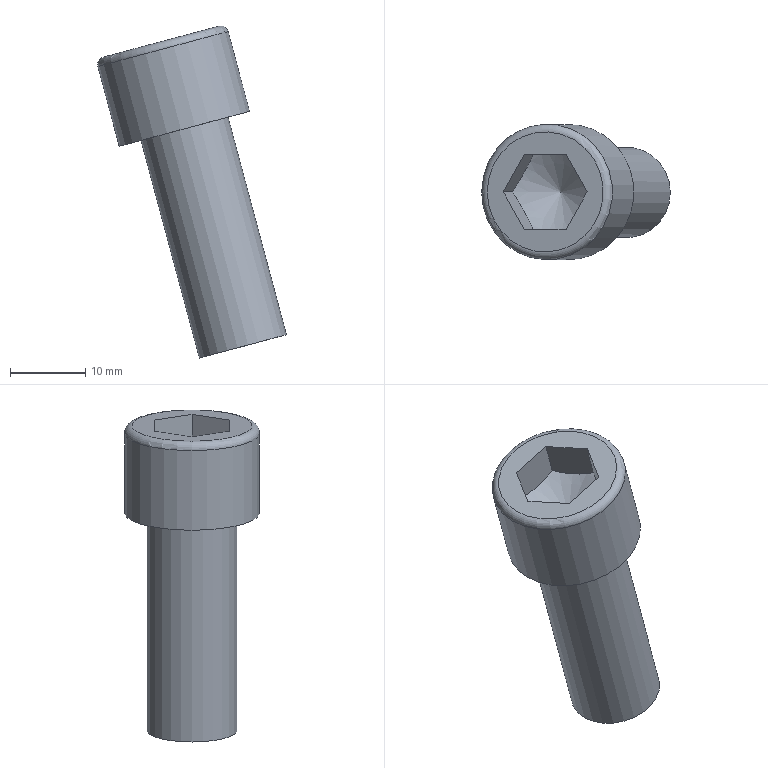Part | NX | features solid 2 | 1 solid | 13 faces | box 25.135 x 18 x 44.226 mm | volume 5917 mm3 | plane 9 | cylinder 2 | cone 1 | torus 1 | commonest cylinder face diameters 12 x1 18 x1
STEP:
#1=CARTESIAN_POINT('',(708.53,850.,-2.528));
#2=VERTEX_POINT('',#1);
#3=CARTESIAN_POINT('',(716.257,850.,-0.4571));
#4=DIRECTION('',(0.2588,0.,-0.9659));
#5=DIRECTION('',(-0.9659,0.,-0.2588));
#6=AXIS2_PLACEMENT_3D('',#3,#4,#5);
#7=CIRCLE('',#6,8.);
#8=EDGE_CURVE('',#2,#2,#7,.T.);
#9=ORIENTED_EDGE('',*,*,#8,.F.);
#10=EDGE_LOOP('',(#9));
#11=FACE_BOUND('',#10,.T.);
#12=CARTESIAN_POINT('',(719.045,845.,0.2901));
#13=VERTEX_POINT('',#12);
#14=CARTESIAN_POINT('',(721.834,850.,1.037));
#15=VERTEX_POINT('',#14);
#16=CARTESIAN_POINT('',(719.045,845.,0.2901));
#17=DIRECTION('',(0.483,0.866,0.1294));
#18=VECTOR('',#17,1000.);
#19=LINE('',#16,#18);
#20=EDGE_CURVE('',#13,#15,#19,.T.);
#21=ORIENTED_EDGE('',*,*,#20,.F.);
#22=CARTESIAN_POINT('',(713.469,845.,-1.204));
#23=VERTEX_POINT('',#22);
#24=CARTESIAN_POINT('',(713.469,845.,-1.204));
#25=DIRECTION('',(0.9659,0.,0.2588));
#26=VECTOR('',#25,1000.);
#27=LINE('',#24,#26);
#28=EDGE_CURVE('',#23,#13,#27,.T.);
#29=ORIENTED_EDGE('',*,*,#28,.F.);
#30=CARTESIAN_POINT('',(710.68,850.,-1.951));
#31=VERTEX_POINT('',#30);
#32=CARTESIAN_POINT('',(710.68,850.,-1.951));
#33=DIRECTION('',(0.483,-0.866,0.1294));
#34=VECTOR('',#33,1000.);
#35=LINE('',#32,#34);
#36=EDGE_CURVE('',#31,#23,#35,.T.);
#37=ORIENTED_EDGE('',*,*,#36,.F.);
#38=CARTESIAN_POINT('',(713.469,855.,-1.204));
#39=VERTEX_POINT('',#38);
#40=CARTESIAN_POINT('',(713.469,855.,-1.204));
#41=DIRECTION('',(-0.483,-0.866,-0.1294));
#42=VECTOR('',#41,1000.);
#43=LINE('',#40,#42);
#44=EDGE_CURVE('',#39,#31,#43,.T.);
#45=ORIENTED_EDGE('',*,*,#44,.F.);
#46=CARTESIAN_POINT('',(719.045,855.,0.2901));
#47=VERTEX_POINT('',#46);
#48=CARTESIAN_POINT('',(719.045,855.,0.2901));
#49=DIRECTION('',(-0.9659,0.,-0.2588));
#50=VECTOR('',#49,1000.);
#51=LINE('',#48,#50);
#52=EDGE_CURVE('',#47,#39,#51,.T.);
#53=ORIENTED_EDGE('',*,*,#52,.F.);
#54=CARTESIAN_POINT('',(721.834,850.,1.037));
#55=DIRECTION('',(-0.483,0.866,-0.1294));
#56=VECTOR('',#55,1000.);
#57=LINE('',#54,#56);
#58=EDGE_CURVE('',#15,#47,#57,.T.);
#59=ORIENTED_EDGE('',*,*,#58,.F.);
#60=EDGE_LOOP('',(#21,#29,#37,#45,#53,#59));
#61=FACE_BOUND('',#60,.T.);
#62=CARTESIAN_POINT('',(716.257,850.,-0.4571));
#63=DIRECTION('',(-0.2588,0.,0.9659));
#64=DIRECTION('',(-0.9659,0.,-0.2588));
#65=AXIS2_PLACEMENT_3D('',#62,#63,#64);
#66=PLANE('',#65);
#67=ADVANCED_FACE('',(#11,#61),#66,.T.);
#68=CARTESIAN_POINT('',(725.158,850.,-10.495));
#69=VERTEX_POINT('',#68);
#70=CARTESIAN_POINT('',(719.363,850.,-12.048));
#71=DIRECTION('',(-0.2588,0.,0.9659));
#72=DIRECTION('',(0.9659,0.,0.2588));
#73=AXIS2_PLACEMENT_3D('',#70,#71,#72);
#74=CIRCLE('',#73,6.);
#75=EDGE_CURVE('',#69,#69,#74,.T.);
#76=ORIENTED_EDGE('',*,*,#75,.T.);
#77=EDGE_LOOP('',(#76));
#78=FACE_BOUND('',#77,.T.);
#79=CARTESIAN_POINT('',(710.67,850.,-14.378));
#80=VERTEX_POINT('',#79);
#81=CARTESIAN_POINT('',(719.363,850.,-12.048));
#82=DIRECTION('',(0.2588,0.,-0.9659));
#83=DIRECTION('',(-0.9659,0.,-0.2588));
#84=AXIS2_PLACEMENT_3D('',#81,#82,#83);
#85=CIRCLE('',#84,9.);
#86=EDGE_CURVE('',#80,#80,#85,.T.);
#87=ORIENTED_EDGE('',*,*,#86,.T.);
#88=EDGE_LOOP('',(#87));
#89=FACE_BOUND('',#88,.T.);
#90=CARTESIAN_POINT('',(719.363,850.,-12.048));
#91=DIRECTION('',(0.2588,0.,-0.9659));
#92=DIRECTION('',(0.9659,0.,0.2588));
#93=AXIS2_PLACEMENT_3D('',#90,#91,#92);
#94=PLANE('',#93);
#95=ADVANCED_FACE('',(#78,#89),#94,.T.);
#96=CARTESIAN_POINT('',(707.823,850.,-3.752));
#97=VERTEX_POINT('',#96);
#98=CARTESIAN_POINT('',(716.516,850.,-1.423));
#99=DIRECTION('',(0.2588,0.,-0.9659));
#100=DIRECTION('',(-0.9659,0.,-0.2588));
#101=AXIS2_PLACEMENT_3D('',#98,#99,#100);
#102=CIRCLE('',#101,9.);
#103=EDGE_CURVE('',#97,#97,#102,.F.);
#104=ORIENTED_EDGE('',*,*,#103,.F.);
#105=EDGE_LOOP('',(#104));
#106=FACE_BOUND('',#105,.T.);
#107=ORIENTED_EDGE('',*,*,#86,.F.);
#108=EDGE_LOOP('',(#107));
#109=FACE_BOUND('',#108,.T.);
#110=CARTESIAN_POINT('',(719.363,850.,-12.048));
#111=DIRECTION('',(-0.2588,0.,0.9659));
#112=DIRECTION('',(-0.9659,0.,-0.2588));
#113=AXIS2_PLACEMENT_3D('',#110,#111,#112);
#114=CYLINDRICAL_SURFACE('',#113,9.);
#115=ADVANCED_FACE('',(#106,#109),#114,.T.);
#116=CARTESIAN_POINT('',(723.042,850.,-3.47));
#117=VERTEX_POINT('',#116);
#118=CARTESIAN_POINT('',(721.834,850.,1.037));
#119=DIRECTION('',(0.2588,0.,-0.9659));
#120=VECTOR('',#119,1000.);
#121=LINE('',#118,#120);
#122=EDGE_CURVE('',#15,#117,#121,.T.);
#123=ORIENTED_EDGE('',*,*,#122,.T.);
#124=CARTESIAN_POINT('',(720.253,845.,-4.218));
#125=VERTEX_POINT('',#124);
#126=CARTESIAN_POINT('',(723.042,850.,-3.47));
#127=CARTESIAN_POINT('',(722.657,849.184,-3.855));
#128=CARTESIAN_POINT('',(721.813,847.509,-4.442));
#129=CARTESIAN_POINT('',(720.78,845.817,-4.359));
#130=CARTESIAN_POINT('',(720.253,845.,-4.218));
#131=B_SPLINE_CURVE_WITH_KNOTS('',3,(#126,#127,#128,#129,#130),.UNSPECIFIED.,.F.,.F.,(4,1,4),(0.000000238,0.002916,0.005831),.UNSPECIFIED.);
#132=EDGE_CURVE('',#117,#125,#131,.T.);
#133=ORIENTED_EDGE('',*,*,#132,.T.);
#134=CARTESIAN_POINT('',(719.045,845.,0.2901));
#135=DIRECTION('',(0.2588,0.,-0.9659));
#136=VECTOR('',#135,1000.);
#137=LINE('',#134,#136);
#138=EDGE_CURVE('',#13,#125,#137,.T.);
#139=ORIENTED_EDGE('',*,*,#138,.F.);
#140=ORIENTED_EDGE('',*,*,#20,.T.);
#141=EDGE_LOOP('',(#123,#133,#139,#140));
#142=FACE_BOUND('',#141,.T.);
#143=CARTESIAN_POINT('',(721.475,847.5,-3.2));
#144=DIRECTION('',(0.8365,-0.5,0.2241));
#145=DIRECTION('',(-0.5215,-0.852,0.04563));
#146=AXIS2_PLACEMENT_3D('',#143,#144,#145);
#147=PLANE('',#146);
#148=ADVANCED_FACE('',(#142),#147,.F.);
#149=ORIENTED_EDGE('',*,*,#138,.T.);
#150=CARTESIAN_POINT('',(714.676,845.,-5.712));
#151=VERTEX_POINT('',#150);
#152=CARTESIAN_POINT('',(720.253,845.,-4.218));
#153=CARTESIAN_POINT('',(719.416,845.,-4.723));
#154=CARTESIAN_POINT('',(717.626,845.,-5.566));
#155=CARTESIAN_POINT('',(715.648,845.,-5.731));
#156=CARTESIAN_POINT('',(714.676,845.,-5.712));
#157=B_SPLINE_CURVE_WITH_KNOTS('',3,(#152,#153,#154,#155,#156),.UNSPECIFIED.,.F.,.F.,(4,1,4),(0.027,0.02987,0.03275),.UNSPECIFIED.);
#158=EDGE_CURVE('',#125,#151,#157,.T.);
#159=ORIENTED_EDGE('',*,*,#158,.T.);
#160=CARTESIAN_POINT('',(713.469,845.,-1.204));
#161=DIRECTION('',(0.2588,0.,-0.9659));
#162=VECTOR('',#161,1000.);
#163=LINE('',#160,#162);
#164=EDGE_CURVE('',#23,#151,#163,.T.);
#165=ORIENTED_EDGE('',*,*,#164,.F.);
#166=ORIENTED_EDGE('',*,*,#28,.T.);
#167=EDGE_LOOP('',(#149,#159,#165,#166));
#168=FACE_BOUND('',#167,.T.);
#169=CARTESIAN_POINT('',(717.292,845.,-4.321));
#170=DIRECTION('',(0.,-1.,0.));
#171=DIRECTION('',(-0.9962,0.,0.08716));
#172=AXIS2_PLACEMENT_3D('',#169,#170,#171);
#173=PLANE('',#172);
#174=ADVANCED_FACE('',(#168),#173,.F.);
#175=ORIENTED_EDGE('',*,*,#164,.T.);
#176=CARTESIAN_POINT('',(711.888,850.,-6.459));
#177=VERTEX_POINT('',#176);
#178=CARTESIAN_POINT('',(714.676,845.,-5.712));
#179=CARTESIAN_POINT('',(714.292,845.816,-6.097));
#180=CARTESIAN_POINT('',(713.448,847.491,-6.684));
#181=CARTESIAN_POINT('',(712.414,849.183,-6.6));
#182=CARTESIAN_POINT('',(711.888,850.,-6.459));
#183=B_SPLINE_CURVE_WITH_KNOTS('',3,(#178,#179,#180,#181,#182),.UNSPECIFIED.,.F.,.F.,(4,1,4),(0.000000238,0.002916,0.005831),.UNSPECIFIED.);
#184=EDGE_CURVE('',#151,#177,#183,.T.);
#185=ORIENTED_EDGE('',*,*,#184,.T.);
#186=CARTESIAN_POINT('',(710.68,850.,-1.951));
#187=DIRECTION('',(0.2588,0.,-0.9659));
#188=VECTOR('',#187,1000.);
#189=LINE('',#186,#188);
#190=EDGE_CURVE('',#31,#177,#189,.T.);
#191=ORIENTED_EDGE('',*,*,#190,.F.);
#192=ORIENTED_EDGE('',*,*,#36,.T.);
#193=EDGE_LOOP('',(#175,#185,#191,#192));
#194=FACE_BOUND('',#193,.T.);
#195=CARTESIAN_POINT('',(713.11,847.5,-5.442));
#196=DIRECTION('',(-0.8365,-0.5,-0.2241));
#197=DIRECTION('',(-0.5215,0.852,0.04563));
#198=AXIS2_PLACEMENT_3D('',#195,#196,#197);
#199=PLANE('',#198);
#200=ADVANCED_FACE('',(#194),#199,.F.);
#201=ORIENTED_EDGE('',*,*,#190,.T.);
#202=CARTESIAN_POINT('',(714.676,855.,-5.712));
#203=VERTEX_POINT('',#202);
#204=CARTESIAN_POINT('',(711.888,850.,-6.459));
#205=CARTESIAN_POINT('',(712.414,850.816,-6.6));
#206=CARTESIAN_POINT('',(713.438,852.491,-6.687));
#207=CARTESIAN_POINT('',(714.291,854.183,-6.097));
#208=CARTESIAN_POINT('',(714.676,855.,-5.712));
#209=B_SPLINE_CURVE_WITH_KNOTS('',3,(#204,#205,#206,#207,#208),.UNSPECIFIED.,.F.,.F.,(4,1,4),(0.000000238,0.002916,0.005831),.UNSPECIFIED.);
#210=EDGE_CURVE('',#177,#203,#209,.T.);
#211=ORIENTED_EDGE('',*,*,#210,.T.);
#212=CARTESIAN_POINT('',(713.469,855.,-1.204));
#213=DIRECTION('',(0.2588,0.,-0.9659));
#214=VECTOR('',#213,1000.);
#215=LINE('',#212,#214);
#216=EDGE_CURVE('',#39,#203,#215,.T.);
#217=ORIENTED_EDGE('',*,*,#216,.F.);
#218=ORIENTED_EDGE('',*,*,#44,.T.);
#219=EDGE_LOOP('',(#201,#211,#217,#218));
#220=FACE_BOUND('',#219,.T.);
#221=CARTESIAN_POINT('',(713.11,852.5,-5.442));
#222=DIRECTION('',(-0.8365,0.5,-0.2241));
#223=DIRECTION('',(0.5215,0.852,-0.04563));
#224=AXIS2_PLACEMENT_3D('',#221,#222,#223);
#225=PLANE('',#224);
#226=ADVANCED_FACE('',(#220),#225,.F.);
#227=ORIENTED_EDGE('',*,*,#216,.T.);
#228=CARTESIAN_POINT('',(720.253,855.,-4.218));
#229=VERTEX_POINT('',#228);
#230=CARTESIAN_POINT('',(720.253,855.,-4.218));
#231=CARTESIAN_POINT('',(719.416,855.,-4.723));
#232=CARTESIAN_POINT('',(717.626,855.,-5.566));
#233=CARTESIAN_POINT('',(715.648,855.,-5.731));
#234=CARTESIAN_POINT('',(714.676,855.,-5.712));
#235=B_SPLINE_CURVE_WITH_KNOTS('',3,(#230,#231,#232,#233,#234),.UNSPECIFIED.,.F.,.F.,(4,1,4),(0.027,0.02987,0.03275),.UNSPECIFIED.);
#236=EDGE_CURVE('',#203,#229,#235,.F.);
#237=ORIENTED_EDGE('',*,*,#236,.T.);
#238=CARTESIAN_POINT('',(719.045,855.,0.2901));
#239=DIRECTION('',(0.2588,0.,-0.9659));
#240=VECTOR('',#239,1000.);
#241=LINE('',#238,#240);
#242=EDGE_CURVE('',#47,#229,#241,.T.);
#243=ORIENTED_EDGE('',*,*,#242,.F.);
#244=ORIENTED_EDGE('',*,*,#52,.T.);
#245=EDGE_LOOP('',(#227,#237,#243,#244));
#246=FACE_BOUND('',#245,.T.);
#247=CARTESIAN_POINT('',(717.292,855.,-4.321));
#248=DIRECTION('',(0.,1.,0.));
#249=DIRECTION('',(0.9962,0.,-0.08716));
#250=AXIS2_PLACEMENT_3D('',#247,#248,#249);
#251=PLANE('',#250);
#252=ADVANCED_FACE('',(#246),#251,.F.);
#253=ORIENTED_EDGE('',*,*,#242,.T.);
#254=CARTESIAN_POINT('',(720.253,855.,-4.218));
#255=CARTESIAN_POINT('',(720.779,854.184,-4.358));
#256=CARTESIAN_POINT('',(721.803,852.509,-4.445));
#257=CARTESIAN_POINT('',(722.656,850.817,-3.856));
#258=CARTESIAN_POINT('',(723.042,850.,-3.47));
#259=B_SPLINE_CURVE_WITH_KNOTS('',3,(#254,#255,#256,#257,#258),.UNSPECIFIED.,.F.,.F.,(4,1,4),(0.000000238,0.002916,0.005831),.UNSPECIFIED.);
#260=EDGE_CURVE('',#229,#117,#259,.T.);
#261=ORIENTED_EDGE('',*,*,#260,.T.);
#262=ORIENTED_EDGE('',*,*,#122,.F.);
#263=ORIENTED_EDGE('',*,*,#58,.T.);
#264=EDGE_LOOP('',(#253,#261,#262,#263));
#265=FACE_BOUND('',#264,.T.);
#266=CARTESIAN_POINT('',(721.475,852.5,-3.2));
#267=DIRECTION('',(0.8365,0.5,0.2241));
#268=DIRECTION('',(0.5215,-0.852,-0.04563));
#269=AXIS2_PLACEMENT_3D('',#266,#267,#268);
#270=PLANE('',#269);
#271=ADVANCED_FACE('',(#265),#270,.F.);
#272=ORIENTED_EDGE('',*,*,#132,.F.);
#273=ORIENTED_EDGE('',*,*,#260,.F.);
#274=ORIENTED_EDGE('',*,*,#236,.F.);
#275=ORIENTED_EDGE('',*,*,#210,.F.);
#276=ORIENTED_EDGE('',*,*,#184,.F.);
#277=ORIENTED_EDGE('',*,*,#158,.F.);
#278=EDGE_LOOP('',(#272,#273,#274,#275,#276,#277));
#279=FACE_BOUND('',#278,.T.);
#280=CARTESIAN_POINT('',(718.328,850.,-8.184));
#281=VERTEX_POINT('',#280);
#282=VERTEX_LOOP('',#281);
#283=FACE_BOUND('',#282,.T.);
#284=CARTESIAN_POINT('',(718.328,850.,-8.184));
#285=DIRECTION('',(-0.2588,0.,0.9659));
#286=DIRECTION('',(-0.9659,0.,-0.2588));
#287=AXIS2_PLACEMENT_3D('',#284,#285,#286);
#288=CONICAL_SURFACE('',#287,0.,1.047);
#289=ADVANCED_FACE('',(#279,#283),#288,.F.);
#290=ORIENTED_EDGE('',*,*,#8,.T.);
#291=EDGE_LOOP('',(#290));
#292=FACE_BOUND('',#291,.T.);
#293=ORIENTED_EDGE('',*,*,#103,.T.);
#294=EDGE_LOOP('',(#293));
#295=FACE_BOUND('',#294,.T.);
#296=CARTESIAN_POINT('',(716.516,850.,-1.423));
#297=DIRECTION('',(-0.2588,0.,0.9659));
#298=DIRECTION('',(-0.9659,0.,-0.2588));
#299=AXIS2_PLACEMENT_3D('',#296,#297,#298);
#300=TOROIDAL_SURFACE('',#299,8.,1.);
#301=ADVANCED_FACE('',(#292,#295),#300,.T.);
#302=CARTESIAN_POINT('',(732.923,850.,-39.473));
#303=VERTEX_POINT('',#302);
#304=CARTESIAN_POINT('',(727.127,850.,-41.026));
#305=DIRECTION('',(-0.2588,0.,0.9659));
#306=DIRECTION('',(0.9659,0.,0.2588));
#307=AXIS2_PLACEMENT_3D('',#304,#305,#306);
#308=CIRCLE('',#307,6.);
#309=EDGE_CURVE('',#303,#303,#308,.F.);
#310=ORIENTED_EDGE('',*,*,#309,.T.);
#311=EDGE_LOOP('',(#310));
#312=FACE_BOUND('',#311,.T.);
#313=CARTESIAN_POINT('',(727.127,850.,-41.026));
#314=DIRECTION('',(0.2588,0.,-0.9659));
#315=DIRECTION('',(0.9659,0.,0.2588));
#316=AXIS2_PLACEMENT_3D('',#313,#314,#315);
#317=PLANE('',#316);
#318=ADVANCED_FACE('',(#312),#317,.T.);
#319=ORIENTED_EDGE('',*,*,#309,.F.);
#320=EDGE_LOOP('',(#319));
#321=FACE_BOUND('',#320,.T.);
#322=ORIENTED_EDGE('',*,*,#75,.F.);
#323=EDGE_LOOP('',(#322));
#324=FACE_BOUND('',#323,.T.);
#325=CARTESIAN_POINT('',(719.363,850.,-12.048));
#326=DIRECTION('',(0.2588,0.,-0.9659));
#327=DIRECTION('',(0.9659,0.,0.2588));
#328=AXIS2_PLACEMENT_3D('',#325,#326,#327);
#329=CYLINDRICAL_SURFACE('',#328,6.);
#330=ADVANCED_FACE('',(#321,#324),#329,.T.);
#331=CLOSED_SHELL('',(#67,#95,#115,#148,#174,#200,#226,#252,#271,#289,#301,#318,#330));
#332=MANIFOLD_SOLID_BREP('',#331);
#333=(LENGTH_UNIT()NAMED_UNIT(*)SI_UNIT(.MILLI.,.METRE.));
#334=UNCERTAINTY_MEASURE_WITH_UNIT(LENGTH_MEASURE(0.0508),#333,'','');
#335=(NAMED_UNIT(*)PLANE_ANGLE_UNIT()SI_UNIT($,.RADIAN.));
#336=(NAMED_UNIT(*)SI_UNIT($,.STERADIAN.)SOLID_ANGLE_UNIT());
#337=(GEOMETRIC_REPRESENTATION_CONTEXT(3)GLOBAL_UNCERTAINTY_ASSIGNED_CONTEXT((#334))GLOBAL_UNIT_ASSIGNED_CONTEXT((#333,#335,#336))REPRESENTATION_CONTEXT('',''));
#338=ADVANCED_BREP_SHAPE_REPRESENTATION('',(#332),#337);